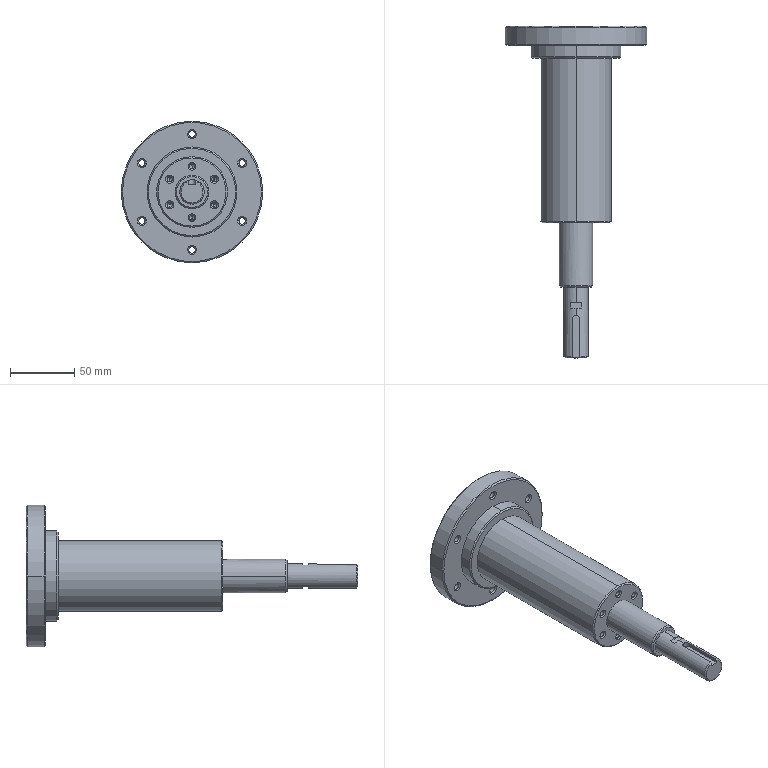Part | STEP file | 05-02 Turntable shaft | 1 solid | 109 faces | box 110 x 258 x 110 mm | volume 522826 mm3 | cone 59 | cylinder 35 | plane 15 | commonest cylinder face diameters 4.2 x12 5 x12 19 x2 26 x2 55 x2 70 x2